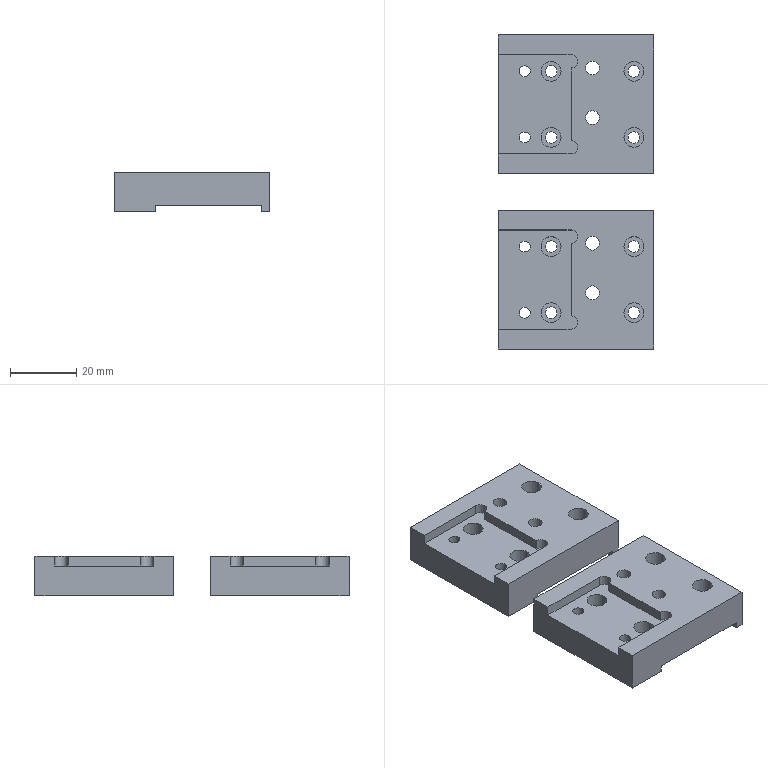NC program | NX | posted with a generic post | part box 47 x 95 x 12 mm
Lines 1 to 1782 of 2681, first 1411 of 1766 lines:
N10 G17 G21 G94 G90
(FLOOR_WALL , TOOL : D80)
N12 T19 M6
N14 G54
N16 G17 G0 G90 X92.5 Y0. S6500 M3
N18 G43 Z30. H19
N20 Z3.
N22 G94 G1 Z0. F1500.
N24 X89.5
N26 X-89.5
N28 X-92.5
N30 Z3.
N32 G0 Z30.
N34 M5
(DRILLING , TOOL : D6A45)
N36 T01 M6
N38 G54
N40 G17 G0 G90 X-36.5 Y-15.5 S5000 M3
N42 G43 Z30. H1
N44 G94 G81 G98 Z-1. F350. R3.
N46 Y-7.5
N48 X-37.5 Y5.
N50 X-36.5 Y17.5
N52 X-16.5
N54 X-22.5 Y5.
N56 X-16.5 Y-7.5
N58 Y-15.5
N60 X16.5
N62 Y-7.5
N64 X15.5 Y5.
N66 X16.5 Y17.5
N68 X36.5
N70 X30.5 Y5.
N72 X36.5 Y-7.5
N74 Y-15.5
N76 G80
N78 G0 X36.5 Y-15.5 Z30.
N80 M5
(DRILLING_COPY_COPY , TOOL : 4.2ZT)
N82 T04 M6
N84 G54
N86 G17 G0 G90 X-37.5 Y5. S2000 M3
N88 G43 Z30. H4
N90 G94 G83 G98 Z-12.762 F300. Q2. R3.
N92 X-22.5
N94 X15.5
N96 X30.5
N98 G80
N100 G0 X30.5 Y5. Z30.
N102 M5
(DRILLING_COPY , TOOL : 3.3ZT)
N104 T03 M6
N106 G54
N108 G17 G0 G90 X-36.5 Y-15.5 S2000 M3
N110 G43 Z30. H3
N112 G94 G83 G98 Z-14.491 F200. Q2. R3.
N114 X-16.5
N116 X16.5
N118 X36.5
N120 G80
N122 G0 X36.5 Y-15.5 Z30.
N124 M5
(DRILLING_COPY_COPY_1 , TOOL : 3.5ZT)
N126 T07 M6
N128 G54
N130 G17 G0 G90 X-16.5 Y-7.5 S2000 M3
N132 G43 Z30. H7
N134 G94 G83 G98 Z-14.052 F200. Q2. R3.
N136 X-36.5
N138 Y17.5
N140 X-16.5
N142 X16.5
N144 X36.5
N146 Y-7.5
N148 X16.5
N150 G80
N152 G0 X16.5 Y-7.5 Z30.
N154 M5
(ZLEVEL_PROFILE , TOOL : D10)
N156 T15 M6
N158 G54
N160 G17 G0 G90 X-0.4 Y-4.832 S9500 M3
N162 G43 Z30. H15
N164 Z1.5
N166 G94 G1 Y-24.054 Z0.493 F1000.
N168 X-0.734 Y-25.398 Z0.42
N170 X-1.416 Y-26.604 Z0.347
N172 X-2.396 Y-27.584 Z0.275
N174 X-3.602 Y-28.266 Z0.202
N176 X-4.946 Y-28.6 Z0.13
N178 X-26.5 Z-1.
N180 X-47.5 F3000.
N182 G2 X-52.6 Y-23.5 R5.1
N184 G1 Y23.5
N186 G2 X-47.5 Y28.6 R5.1
N188 G1 X-5.5
N190 G2 X-0.4 Y23.5 R5.1
N192 G1 Y-23.5
N194 G2 X-5.5 Y-28.6 R5.1
N196 G1 X-26.5
N198 X-47.5 Z-1.1
N200 X-48. Y-28.575 Z-1.102
N202 X-48.495 Y-28.502 Z-1.105
N204 X-48.98 Y-28.38 Z-1.107
N206 X-49.452 Y-28.212 Z-1.11
N208 X-49.904 Y-27.998 Z-1.112
N210 X-50.333 Y-27.74 Z-1.114
N212 X-50.735 Y-27.442 Z-1.117
N214 X-51.106 Y-27.106 Z-1.119
N216 X-51.442 Y-26.735 Z-1.121
N218 X-51.74 Y-26.333 Z-1.124
N220 X-51.998 Y-25.904 Z-1.126
N222 X-52.212 Y-25.452 Z-1.129
N224 X-52.38 Y-24.98 Z-1.131
N226 X-52.502 Y-24.495 Z-1.133
N228 X-52.575 Y-24. Z-1.136
N230 X-52.6 Y-23.5 Z-1.138
N232 Y23.5 Z-1.362
N234 X-52.575 Y24. Z-1.364
N236 X-52.502 Y24.495 Z-1.367
N238 X-52.38 Y24.98 Z-1.369
N240 X-52.212 Y25.452 Z-1.371
N242 X-51.998 Y25.904 Z-1.374
N244 X-51.74 Y26.333 Z-1.376
N246 X-51.442 Y26.735 Z-1.379
N248 X-51.106 Y27.106 Z-1.381
N250 X-50.735 Y27.442 Z-1.383
N252 X-50.333 Y27.74 Z-1.386
N254 X-49.904 Y27.998 Z-1.388
N256 X-49.452 Y28.212 Z-1.39
N258 X-48.98 Y28.38 Z-1.393
N260 X-48.495 Y28.502 Z-1.395
N262 X-48. Y28.575 Z-1.398
N264 X-47.5 Y28.6 Z-1.4
N266 X-5.5 Z-1.6
N268 X-5. Y28.575 Z-1.602
N270 X-4.505 Y28.502 Z-1.605
N272 X-4.02 Y28.38 Z-1.607
N274 X-3.548 Y28.212 Z-1.61
N276 X-3.096 Y27.998 Z-1.612
N278 X-2.667 Y27.74 Z-1.614
N280 X-2.265 Y27.442 Z-1.617
N282 X-1.894 Y27.106 Z-1.619
N284 X-1.558 Y26.735 Z-1.621
N286 X-1.26 Y26.333 Z-1.624
N288 X-1.002 Y25.904 Z-1.626
N290 X-0.788 Y25.452 Z-1.629
N292 X-0.62 Y24.98 Z-1.631
N294 X-0.498 Y24.495 Z-1.633
N296 X-0.425 Y24. Z-1.636
N298 X-0.4 Y23.5 Z-1.638
N300 Y-23.5 Z-1.862
N302 X-0.425 Y-24. Z-1.864
N304 X-0.498 Y-24.495 Z-1.867
N306 X-0.62 Y-24.98 Z-1.869
N308 X-0.788 Y-25.452 Z-1.871
N310 X-1.002 Y-25.904 Z-1.874
N312 X-1.26 Y-26.333 Z-1.876
N314 X-1.558 Y-26.735 Z-1.879
N316 X-1.894 Y-27.106 Z-1.881
N318 X-2.265 Y-27.442 Z-1.883
N320 X-2.667 Y-27.74 Z-1.886
N322 X-3.096 Y-27.998 Z-1.888
N324 X-3.548 Y-28.212 Z-1.89
N326 X-4.02 Y-28.38 Z-1.893
N328 X-4.505 Y-28.502 Z-1.895
N330 X-5. Y-28.575 Z-1.898
N332 X-5.5 Y-28.6 Z-1.9
N334 X-26.5 Z-2.
N336 X-47.5 Z-2.1
N338 X-48. Y-28.575 Z-2.102
N340 X-48.495 Y-28.502 Z-2.105
N342 X-48.98 Y-28.38 Z-2.107
N344 X-49.452 Y-28.212 Z-2.11
N346 X-49.904 Y-27.998 Z-2.112
N348 X-50.333 Y-27.74 Z-2.114
N350 X-50.735 Y-27.442 Z-2.117
N352 X-51.106 Y-27.106 Z-2.119
N354 X-51.442 Y-26.735 Z-2.121
N356 X-51.74 Y-26.333 Z-2.124
N358 X-51.998 Y-25.904 Z-2.126
N360 X-52.212 Y-25.452 Z-2.129
N362 X-52.38 Y-24.98 Z-2.131
N364 X-52.502 Y-24.495 Z-2.133
N366 X-52.575 Y-24. Z-2.136
N368 X-52.6 Y-23.5 Z-2.138
N370 Y23.5 Z-2.362
N372 X-52.575 Y24. Z-2.364
N374 X-52.502 Y24.495 Z-2.367
N376 X-52.38 Y24.98 Z-2.369
N378 X-52.212 Y25.452 Z-2.371
N380 X-51.998 Y25.904 Z-2.374
N382 X-51.74 Y26.333 Z-2.376
N384 X-51.442 Y26.735 Z-2.379
N386 X-51.106 Y27.106 Z-2.381
N388 X-50.735 Y27.442 Z-2.383
N390 X-50.333 Y27.74 Z-2.386
N392 X-49.904 Y27.998 Z-2.388
N394 X-49.452 Y28.212 Z-2.39
N396 X-48.98 Y28.38 Z-2.393
N398 X-48.495 Y28.502 Z-2.395
N400 X-48. Y28.575 Z-2.398
N402 X-47.5 Y28.6 Z-2.4
N404 X-5.5 Z-2.6
N406 X-5. Y28.575 Z-2.602
N408 X-4.505 Y28.502 Z-2.605
N410 X-4.02 Y28.38 Z-2.607
N412 X-3.548 Y28.212 Z-2.61
N414 X-3.096 Y27.998 Z-2.612
N416 X-2.667 Y27.74 Z-2.614
N418 X-2.265 Y27.442 Z-2.617
N420 X-1.894 Y27.106 Z-2.619
N422 X-1.558 Y26.735 Z-2.621
N424 X-1.26 Y26.333 Z-2.624
N426 X-1.002 Y25.904 Z-2.626
N428 X-0.788 Y25.452 Z-2.629
N430 X-0.62 Y24.98 Z-2.631
N432 X-0.498 Y24.495 Z-2.633
N434 X-0.425 Y24. Z-2.636
N436 X-0.4 Y23.5 Z-2.638
N438 Y-23.5 Z-2.862
N440 X-0.425 Y-24. Z-2.864
N442 X-0.498 Y-24.495 Z-2.867
N444 X-0.62 Y-24.98 Z-2.869
N446 X-0.788 Y-25.452 Z-2.871
N448 X-1.002 Y-25.904 Z-2.874
N450 X-1.26 Y-26.333 Z-2.876
N452 X-1.558 Y-26.735 Z-2.879
N454 X-1.894 Y-27.106 Z-2.881
N456 X-2.265 Y-27.442 Z-2.883
N458 X-2.667 Y-27.74 Z-2.886
N460 X-3.096 Y-27.998 Z-2.888
N462 X-3.548 Y-28.212 Z-2.89
N464 X-4.02 Y-28.38 Z-2.893
N466 X-4.505 Y-28.502 Z-2.895
N468 X-5. Y-28.575 Z-2.898
N470 X-5.5 Y-28.6 Z-2.9
N472 X-26.5 Z-3.
N474 X-47.5 Z-3.1
N476 X-48. Y-28.575 Z-3.102
N478 X-48.495 Y-28.502 Z-3.105
N480 X-48.98 Y-28.38 Z-3.107
N482 X-49.452 Y-28.212 Z-3.11
N484 X-49.904 Y-27.998 Z-3.112
N486 X-50.333 Y-27.74 Z-3.114
N488 X-50.735 Y-27.442 Z-3.117
N490 X-51.106 Y-27.106 Z-3.119
N492 X-51.442 Y-26.735 Z-3.121
N494 X-51.74 Y-26.333 Z-3.124
N496 X-51.998 Y-25.904 Z-3.126
N498 X-52.212 Y-25.452 Z-3.129
N500 X-52.38 Y-24.98 Z-3.131
N502 X-52.502 Y-24.495 Z-3.133
N504 X-52.575 Y-24. Z-3.136
N506 X-52.6 Y-23.5 Z-3.138
N508 Y23.5 Z-3.362
N510 X-52.575 Y24. Z-3.364
N512 X-52.502 Y24.495 Z-3.367
N514 X-52.38 Y24.98 Z-3.369
N516 X-52.212 Y25.452 Z-3.371
N518 X-51.998 Y25.904 Z-3.374
N520 X-51.74 Y26.333 Z-3.376
N522 X-51.442 Y26.735 Z-3.379
N524 X-51.106 Y27.106 Z-3.381
N526 X-50.735 Y27.442 Z-3.383
N528 X-50.333 Y27.74 Z-3.386
N530 X-49.904 Y27.998 Z-3.388
N532 X-49.452 Y28.212 Z-3.39
N534 X-48.98 Y28.38 Z-3.393
N536 X-48.495 Y28.502 Z-3.395
N538 X-48. Y28.575 Z-3.398
N540 X-47.5 Y28.6 Z-3.4
N542 X-5.5 Z-3.6
N544 X-5. Y28.575 Z-3.602
N546 X-4.505 Y28.502 Z-3.605
N548 X-4.02 Y28.38 Z-3.607
N550 X-3.548 Y28.212 Z-3.61
N552 X-3.096 Y27.998 Z-3.612
N554 X-2.667 Y27.74 Z-3.614
N556 X-2.265 Y27.442 Z-3.617
N558 X-1.894 Y27.106 Z-3.619
N560 X-1.558 Y26.735 Z-3.621
N562 X-1.26 Y26.333 Z-3.624
N564 X-1.002 Y25.904 Z-3.626
N566 X-0.788 Y25.452 Z-3.629
N568 X-0.62 Y24.98 Z-3.631
N570 X-0.498 Y24.495 Z-3.633
N572 X-0.425 Y24. Z-3.636
N574 X-0.4 Y23.5 Z-3.638
N576 Y-23.5 Z-3.862
N578 X-0.425 Y-24. Z-3.864
N580 X-0.498 Y-24.495 Z-3.867
N582 X-0.62 Y-24.98 Z-3.869
N584 X-0.788 Y-25.452 Z-3.871
N586 X-1.002 Y-25.904 Z-3.874
N588 X-1.26 Y-26.333 Z-3.876
N590 X-1.558 Y-26.735 Z-3.879
N592 X-1.894 Y-27.106 Z-3.881
N594 X-2.265 Y-27.442 Z-3.883
N596 X-2.667 Y-27.74 Z-3.886
N598 X-3.096 Y-27.998 Z-3.888
N600 X-3.548 Y-28.212 Z-3.89
N602 X-4.02 Y-28.38 Z-3.893
N604 X-4.505 Y-28.502 Z-3.895
N606 X-5. Y-28.575 Z-3.898
N608 X-5.5 Y-28.6 Z-3.9
N610 X-26.5 Z-4.
N612 X-47.5 Z-4.1
N614 X-48. Y-28.575 Z-4.102
N616 X-48.495 Y-28.502 Z-4.105
N618 X-48.98 Y-28.38 Z-4.107
N620 X-49.452 Y-28.212 Z-4.11
N622 X-49.904 Y-27.998 Z-4.112
N624 X-50.333 Y-27.74 Z-4.114
N626 X-50.735 Y-27.442 Z-4.117
N628 X-51.106 Y-27.106 Z-4.119
N630 X-51.442 Y-26.735 Z-4.121
N632 X-51.74 Y-26.333 Z-4.124
N634 X-51.998 Y-25.904 Z-4.126
N636 X-52.212 Y-25.452 Z-4.129
N638 X-52.38 Y-24.98 Z-4.131
N640 X-52.502 Y-24.495 Z-4.133
N642 X-52.575 Y-24. Z-4.136
N644 X-52.6 Y-23.5 Z-4.138
N646 Y23.5 Z-4.362
N648 X-52.575 Y24. Z-4.364
N650 X-52.502 Y24.495 Z-4.367
N652 X-52.38 Y24.98 Z-4.369
N654 X-52.212 Y25.452 Z-4.371
N656 X-51.998 Y25.904 Z-4.374
N658 X-51.74 Y26.333 Z-4.376
N660 X-51.442 Y26.735 Z-4.379
N662 X-51.106 Y27.106 Z-4.381
N664 X-50.735 Y27.442 Z-4.383
N666 X-50.333 Y27.74 Z-4.386
N668 X-49.904 Y27.998 Z-4.388
N670 X-49.452 Y28.212 Z-4.39
N672 X-48.98 Y28.38 Z-4.393
N674 X-48.495 Y28.502 Z-4.395
N676 X-48. Y28.575 Z-4.398
N678 X-47.5 Y28.6 Z-4.4
N680 X-5.5 Z-4.6
N682 X-5. Y28.575 Z-4.602
N684 X-4.505 Y28.502 Z-4.605
N686 X-4.02 Y28.38 Z-4.607
N688 X-3.548 Y28.212 Z-4.61
N690 X-3.096 Y27.998 Z-4.612
N692 X-2.667 Y27.74 Z-4.614
N694 X-2.265 Y27.442 Z-4.617
N696 X-1.894 Y27.106 Z-4.619
N698 X-1.558 Y26.735 Z-4.621
N700 X-1.26 Y26.333 Z-4.624
N702 X-1.002 Y25.904 Z-4.626
N704 X-0.788 Y25.452 Z-4.629
N706 X-0.62 Y24.98 Z-4.631
N708 X-0.498 Y24.495 Z-4.633
N710 X-0.425 Y24. Z-4.636
N712 X-0.4 Y23.5 Z-4.638
N714 Y-23.5 Z-4.862
N716 X-0.425 Y-24. Z-4.864
N718 X-0.498 Y-24.495 Z-4.867
N720 X-0.62 Y-24.98 Z-4.869
N722 X-0.788 Y-25.452 Z-4.871
N724 X-1.002 Y-25.904 Z-4.874
N726 X-1.26 Y-26.333 Z-4.876
N728 X-1.558 Y-26.735 Z-4.879
N730 X-1.894 Y-27.106 Z-4.881
N732 X-2.265 Y-27.442 Z-4.883
N734 X-2.667 Y-27.74 Z-4.886
N736 X-3.096 Y-27.998 Z-4.888
N738 X-3.548 Y-28.212 Z-4.89
N740 X-4.02 Y-28.38 Z-4.893
N742 X-4.505 Y-28.502 Z-4.895
N744 X-5. Y-28.575 Z-4.898
N746 X-5.5 Y-28.6 Z-4.9
N748 X-26.5 Z-5.
N750 X-47.5 Z-5.1
N752 X-48. Y-28.575 Z-5.102
N754 X-48.495 Y-28.502 Z-5.105
N756 X-48.98 Y-28.38 Z-5.107
N758 X-49.452 Y-28.212 Z-5.11
N760 X-49.904 Y-27.998 Z-5.112
N762 X-50.333 Y-27.74 Z-5.114
N764 X-50.735 Y-27.442 Z-5.117
N766 X-51.106 Y-27.106 Z-5.119
N768 X-51.442 Y-26.735 Z-5.121
N770 X-51.74 Y-26.333 Z-5.124
N772 X-51.998 Y-25.904 Z-5.126
N774 X-52.212 Y-25.452 Z-5.129
N776 X-52.38 Y-24.98 Z-5.131
N778 X-52.502 Y-24.495 Z-5.133
N780 X-52.575 Y-24. Z-5.136
N782 X-52.6 Y-23.5 Z-5.138
N784 Y23.5 Z-5.362
N786 X-52.575 Y24. Z-5.364
N788 X-52.502 Y24.495 Z-5.367
N790 X-52.38 Y24.98 Z-5.369
N792 X-52.212 Y25.452 Z-5.371
N794 X-51.998 Y25.904 Z-5.374
N796 X-51.74 Y26.333 Z-5.376
N798 X-51.442 Y26.735 Z-5.379
N800 X-51.106 Y27.106 Z-5.381
N802 X-50.735 Y27.442 Z-5.383
N804 X-50.333 Y27.74 Z-5.386
N806 X-49.904 Y27.998 Z-5.388
N808 X-49.452 Y28.212 Z-5.39
N810 X-48.98 Y28.38 Z-5.393
N812 X-48.495 Y28.502 Z-5.395
N814 X-48. Y28.575 Z-5.398
N816 X-47.5 Y28.6 Z-5.4
N818 X-5.5 Z-5.6
N820 X-5. Y28.575 Z-5.602
N822 X-4.505 Y28.502 Z-5.605
N824 X-4.02 Y28.38 Z-5.607
N826 X-3.548 Y28.212 Z-5.61
N828 X-3.096 Y27.998 Z-5.612
N830 X-2.667 Y27.74 Z-5.614
N832 X-2.265 Y27.442 Z-5.617
N834 X-1.894 Y27.106 Z-5.619
N836 X-1.558 Y26.735 Z-5.621
N838 X-1.26 Y26.333 Z-5.624
N840 X-1.002 Y25.904 Z-5.626
N842 X-0.788 Y25.452 Z-5.629
N844 X-0.62 Y24.98 Z-5.631
N846 X-0.498 Y24.495 Z-5.633
N848 X-0.425 Y24. Z-5.636
N850 X-0.4 Y23.5 Z-5.638
N852 Y-23.5 Z-5.862
N854 X-0.425 Y-24. Z-5.864
N856 X-0.498 Y-24.495 Z-5.867
N858 X-0.62 Y-24.98 Z-5.869
N860 X-0.788 Y-25.452 Z-5.871
N862 X-1.002 Y-25.904 Z-5.874
N864 X-1.26 Y-26.333 Z-5.876
N866 X-1.558 Y-26.735 Z-5.879
N868 X-1.894 Y-27.106 Z-5.881
N870 X-2.265 Y-27.442 Z-5.883
N872 X-2.667 Y-27.74 Z-5.886
N874 X-3.096 Y-27.998 Z-5.888
N876 X-3.548 Y-28.212 Z-5.89
N878 X-4.02 Y-28.38 Z-5.893
N880 X-4.505 Y-28.502 Z-5.895
N882 X-5. Y-28.575 Z-5.898
N884 X-5.5 Y-28.6 Z-5.9
N886 X-26.5 Z-6.
N888 X-47.5 Z-6.1
N890 X-48. Y-28.575 Z-6.102
N892 X-48.495 Y-28.502 Z-6.105
N894 X-48.98 Y-28.38 Z-6.107
N896 X-49.452 Y-28.212 Z-6.11
N898 X-49.904 Y-27.998 Z-6.112
N900 X-50.333 Y-27.74 Z-6.114
N902 X-50.735 Y-27.442 Z-6.117
N904 X-51.106 Y-27.106 Z-6.119
N906 X-51.442 Y-26.735 Z-6.121
N908 X-51.74 Y-26.333 Z-6.124
N910 X-51.998 Y-25.904 Z-6.126
N912 X-52.212 Y-25.452 Z-6.129
N914 X-52.38 Y-24.98 Z-6.131
N916 X-52.502 Y-24.495 Z-6.133
N918 X-52.575 Y-24. Z-6.136
N920 X-52.6 Y-23.5 Z-6.138
N922 Y23.5 Z-6.362
N924 X-52.575 Y24. Z-6.364
N926 X-52.502 Y24.495 Z-6.367
N928 X-52.38 Y24.98 Z-6.369
N930 X-52.212 Y25.452 Z-6.371
N932 X-51.998 Y25.904 Z-6.374
N934 X-51.74 Y26.333 Z-6.376
N936 X-51.442 Y26.735 Z-6.379
N938 X-51.106 Y27.106 Z-6.381
N940 X-50.735 Y27.442 Z-6.383
N942 X-50.333 Y27.74 Z-6.386
N944 X-49.904 Y27.998 Z-6.388
N946 X-49.452 Y28.212 Z-6.39
N948 X-48.98 Y28.38 Z-6.393
N950 X-48.495 Y28.502 Z-6.395
N952 X-48. Y28.575 Z-6.398
N954 X-47.5 Y28.6 Z-6.4
N956 X-5.5 Z-6.6
N958 X-5. Y28.575 Z-6.602
N960 X-4.505 Y28.502 Z-6.605
N962 X-4.02 Y28.38 Z-6.607
N964 X-3.548 Y28.212 Z-6.61
N966 X-3.096 Y27.998 Z-6.612
N968 X-2.667 Y27.74 Z-6.614
N970 X-2.265 Y27.442 Z-6.617
N972 X-1.894 Y27.106 Z-6.619
N974 X-1.558 Y26.735 Z-6.621
N976 X-1.26 Y26.333 Z-6.624
N978 X-1.002 Y25.904 Z-6.626
N980 X-0.788 Y25.452 Z-6.629
N982 X-0.62 Y24.98 Z-6.631
N984 X-0.498 Y24.495 Z-6.633
N986 X-0.425 Y24. Z-6.636
N988 X-0.4 Y23.5 Z-6.638
N990 Y-23.5 Z-6.862
N992 X-0.425 Y-24. Z-6.864
N994 X-0.498 Y-24.495 Z-6.867
N996 X-0.62 Y-24.98 Z-6.869
N998 X-0.788 Y-25.452 Z-6.871
N1000 X-1.002 Y-25.904 Z-6.874
N1002 X-1.26 Y-26.333 Z-6.876
N1004 X-1.558 Y-26.735 Z-6.879
N1006 X-1.894 Y-27.106 Z-6.881
N1008 X-2.265 Y-27.442 Z-6.883
N1010 X-2.667 Y-27.74 Z-6.886
N1012 X-3.096 Y-27.998 Z-6.888
N1014 X-3.548 Y-28.212 Z-6.89
N1016 X-4.02 Y-28.38 Z-6.893
N1018 X-4.505 Y-28.502 Z-6.895
N1020 X-5. Y-28.575 Z-6.898
N1022 X-5.5 Y-28.6 Z-6.9
N1024 X-26.5 Z-7.
N1026 X-47.5 Z-7.1
N1028 X-48. Y-28.575 Z-7.102
N1030 X-48.495 Y-28.502 Z-7.105
N1032 X-48.98 Y-28.38 Z-7.107
N1034 X-49.452 Y-28.212 Z-7.11
N1036 X-49.904 Y-27.998 Z-7.112
N1038 X-50.333 Y-27.74 Z-7.114
N1040 X-50.735 Y-27.442 Z-7.117
N1042 X-51.106 Y-27.106 Z-7.119
N1044 X-51.442 Y-26.735 Z-7.121
N1046 X-51.74 Y-26.333 Z-7.124
N1048 X-51.998 Y-25.904 Z-7.126
N1050 X-52.212 Y-25.452 Z-7.129
N1052 X-52.38 Y-24.98 Z-7.131
N1054 X-52.502 Y-24.495 Z-7.133
N1056 X-52.575 Y-24. Z-7.136
N1058 X-52.6 Y-23.5 Z-7.138
N1060 Y23.5 Z-7.362
N1062 X-52.575 Y24. Z-7.364
N1064 X-52.502 Y24.495 Z-7.367
N1066 X-52.38 Y24.98 Z-7.369
N1068 X-52.212 Y25.452 Z-7.371
N1070 X-51.998 Y25.904 Z-7.374
N1072 X-51.74 Y26.333 Z-7.376
N1074 X-51.442 Y26.735 Z-7.379
N1076 X-51.106 Y27.106 Z-7.381
N1078 X-50.735 Y27.442 Z-7.383
N1080 X-50.333 Y27.74 Z-7.386
N1082 X-49.904 Y27.998 Z-7.388
N1084 X-49.452 Y28.212 Z-7.39
N1086 X-48.98 Y28.38 Z-7.393
N1088 X-48.495 Y28.502 Z-7.395
N1090 X-48. Y28.575 Z-7.398
N1092 X-47.5 Y28.6 Z-7.4
N1094 X-5.5 Z-7.6
N1096 X-5. Y28.575 Z-7.602
N1098 X-4.505 Y28.502 Z-7.605
N1100 X-4.02 Y28.38 Z-7.607
N1102 X-3.548 Y28.212 Z-7.61
N1104 X-3.096 Y27.998 Z-7.612
N1106 X-2.667 Y27.74 Z-7.614
N1108 X-2.265 Y27.442 Z-7.617
N1110 X-1.894 Y27.106 Z-7.619
N1112 X-1.558 Y26.735 Z-7.621
N1114 X-1.26 Y26.333 Z-7.624
N1116 X-1.002 Y25.904 Z-7.626
N1118 X-0.788 Y25.452 Z-7.629
N1120 X-0.62 Y24.98 Z-7.631
N1122 X-0.498 Y24.495 Z-7.633
N1124 X-0.425 Y24. Z-7.636
N1126 X-0.4 Y23.5 Z-7.638
N1128 Y-23.5 Z-7.862
N1130 X-0.425 Y-24. Z-7.864
N1132 X-0.498 Y-24.495 Z-7.867
N1134 X-0.62 Y-24.98 Z-7.869
N1136 X-0.788 Y-25.452 Z-7.871
N1138 X-1.002 Y-25.904 Z-7.874
N1140 X-1.26 Y-26.333 Z-7.876
N1142 X-1.558 Y-26.735 Z-7.879
N1144 X-1.894 Y-27.106 Z-7.881
N1146 X-2.265 Y-27.442 Z-7.883
N1148 X-2.667 Y-27.74 Z-7.886
N1150 X-3.096 Y-27.998 Z-7.888
N1152 X-3.548 Y-28.212 Z-7.89
N1154 X-4.02 Y-28.38 Z-7.893
N1156 X-4.505 Y-28.502 Z-7.895
N1158 X-5. Y-28.575 Z-7.898
N1160 X-5.5 Y-28.6 Z-7.9
N1162 X-26.5 Z-8.
N1164 X-47.5 Z-8.1
N1166 X-48. Y-28.575 Z-8.102
N1168 X-48.495 Y-28.502 Z-8.105
N1170 X-48.98 Y-28.38 Z-8.107
N1172 X-49.452 Y-28.212 Z-8.11
N1174 X-49.904 Y-27.998 Z-8.112
N1176 X-50.333 Y-27.74 Z-8.114
N1178 X-50.735 Y-27.442 Z-8.117
N1180 X-51.106 Y-27.106 Z-8.119
N1182 X-51.442 Y-26.735 Z-8.121
N1184 X-51.74 Y-26.333 Z-8.124
N1186 X-51.998 Y-25.904 Z-8.126
N1188 X-52.212 Y-25.452 Z-8.129
N1190 X-52.38 Y-24.98 Z-8.131
N1192 X-52.502 Y-24.495 Z-8.133
N1194 X-52.575 Y-24. Z-8.136
N1196 X-52.6 Y-23.5 Z-8.138
N1198 Y23.5 Z-8.362
N1200 X-52.575 Y24. Z-8.364
N1202 X-52.502 Y24.495 Z-8.367
N1204 X-52.38 Y24.98 Z-8.369
N1206 X-52.212 Y25.452 Z-8.371
N1208 X-51.998 Y25.904 Z-8.374
N1210 X-51.74 Y26.333 Z-8.376
N1212 X-51.442 Y26.735 Z-8.379
N1214 X-51.106 Y27.106 Z-8.381
N1216 X-50.735 Y27.442 Z-8.383
N1218 X-50.333 Y27.74 Z-8.386
N1220 X-49.904 Y27.998 Z-8.388
N1222 X-49.452 Y28.212 Z-8.39
N1224 X-48.98 Y28.38 Z-8.393
N1226 X-48.495 Y28.502 Z-8.395
N1228 X-48. Y28.575 Z-8.398
N1230 X-47.5 Y28.6 Z-8.4
N1232 X-5.5 Z-8.6
N1234 X-5. Y28.575 Z-8.602
N1236 X-4.505 Y28.502 Z-8.605
N1238 X-4.02 Y28.38 Z-8.607
N1240 X-3.548 Y28.212 Z-8.61
N1242 X-3.096 Y27.998 Z-8.612
N1244 X-2.667 Y27.74 Z-8.614
N1246 X-2.265 Y27.442 Z-8.617
N1248 X-1.894 Y27.106 Z-8.619
N1250 X-1.558 Y26.735 Z-8.621
N1252 X-1.26 Y26.333 Z-8.624
N1254 X-1.002 Y25.904 Z-8.626
N1256 X-0.788 Y25.452 Z-8.629
N1258 X-0.62 Y24.98 Z-8.631
N1260 X-0.498 Y24.495 Z-8.633
N1262 X-0.425 Y24. Z-8.636
N1264 X-0.4 Y23.5 Z-8.638
N1266 Y-23.5 Z-8.862
N1268 X-0.425 Y-24. Z-8.864
N1270 X-0.498 Y-24.495 Z-8.867
N1272 X-0.62 Y-24.98 Z-8.869
N1274 X-0.788 Y-25.452 Z-8.871
N1276 X-1.002 Y-25.904 Z-8.874
N1278 X-1.26 Y-26.333 Z-8.876
N1280 X-1.558 Y-26.735 Z-8.879
N1282 X-1.894 Y-27.106 Z-8.881
N1284 X-2.265 Y-27.442 Z-8.883
N1286 X-2.667 Y-27.74 Z-8.886
N1288 X-3.096 Y-27.998 Z-8.888
N1290 X-3.548 Y-28.212 Z-8.89
N1292 X-4.02 Y-28.38 Z-8.893
N1294 X-4.505 Y-28.502 Z-8.895
N1296 X-5. Y-28.575 Z-8.898
N1298 X-5.5 Y-28.6 Z-8.9
N1300 X-26.5 Z-9.
N1302 X-47.5 Z-9.1
N1304 X-48. Y-28.575 Z-9.102
N1306 X-48.495 Y-28.502 Z-9.105
N1308 X-48.98 Y-28.38 Z-9.107
N1310 X-49.452 Y-28.212 Z-9.11
N1312 X-49.904 Y-27.998 Z-9.112
N1314 X-50.333 Y-27.74 Z-9.114
N1316 X-50.735 Y-27.442 Z-9.117
N1318 X-51.106 Y-27.106 Z-9.119
N1320 X-51.442 Y-26.735 Z-9.121
N1322 X-51.74 Y-26.333 Z-9.124
N1324 X-51.998 Y-25.904 Z-9.126
N1326 X-52.212 Y-25.452 Z-9.129
N1328 X-52.38 Y-24.98 Z-9.131
N1330 X-52.502 Y-24.495 Z-9.133
N1332 X-52.575 Y-24. Z-9.136
N1334 X-52.6 Y-23.5 Z-9.138
N1336 Y23.5 Z-9.362
N1338 X-52.575 Y24. Z-9.364
N1340 X-52.502 Y24.495 Z-9.367
N1342 X-52.38 Y24.98 Z-9.369
N1344 X-52.212 Y25.452 Z-9.371
N1346 X-51.998 Y25.904 Z-9.374
N1348 X-51.74 Y26.333 Z-9.376
N1350 X-51.442 Y26.735 Z-9.379
N1352 X-51.106 Y27.106 Z-9.381
N1354 X-50.735 Y27.442 Z-9.383
N1356 X-50.333 Y27.74 Z-9.386
N1358 X-49.904 Y27.998 Z-9.388
N1360 X-49.452 Y28.212 Z-9.39
N1362 X-48.98 Y28.38 Z-9.393
N1364 X-48.495 Y28.502 Z-9.395
N1366 X-48. Y28.575 Z-9.398
N1368 X-47.5 Y28.6 Z-9.4
N1370 X-5.5 Z-9.6
N1372 X-5. Y28.575 Z-9.602
N1374 X-4.505 Y28.502 Z-9.605
N1376 X-4.02 Y28.38 Z-9.607
N1378 X-3.548 Y28.212 Z-9.61
N1380 X-3.096 Y27.998 Z-9.612
N1382 X-2.667 Y27.74 Z-9.614
N1384 X-2.265 Y27.442 Z-9.617
N1386 X-1.894 Y27.106 Z-9.619
N1388 X-1.558 Y26.735 Z-9.621
N1390 X-1.26 Y26.333 Z-9.624
N1392 X-1.002 Y25.904 Z-9.626
N1394 X-0.788 Y25.452 Z-9.629
N1396 X-0.62 Y24.98 Z-9.631
N1398 X-0.498 Y24.495 Z-9.633
N1400 X-0.425 Y24. Z-9.636
N1402 X-0.4 Y23.5 Z-9.638
N1404 Y-23.5 Z-9.862
N1406 X-0.425 Y-24. Z-9.864
N1408 X-0.498 Y-24.495 Z-9.867
N1410 X-0.62 Y-24.98 Z-9.869
N1412 X-0.788 Y-25.452 Z-9.871
N1414 X-1.002 Y-25.904 Z-9.874
N1416 X-1.26 Y-26.333 Z-9.876
N1418 X-1.558 Y-26.735 Z-9.879
N1420 X-1.894 Y-27.106 Z-9.881
N1422 X-2.265 Y-27.442 Z-9.883
N1424 X-2.667 Y-27.74 Z-9.886
N1426 X-3.096 Y-27.998 Z-9.888
N1428 X-3.548 Y-28.212 Z-9.89
N1430 X-4.02 Y-28.38 Z-9.893
N1432 X-4.505 Y-28.502 Z-9.895
N1434 X-5. Y-28.575 Z-9.898
N1436 X-5.5 Y-28.6 Z-9.9
N1438 X-26.5 Z-10.
N1440 X-47.5 Z-10.1
N1442 X-48. Y-28.575 Z-10.102
N1444 X-48.495 Y-28.502 Z-10.105
N1446 X-48.98 Y-28.38 Z-10.107
N1448 X-49.452 Y-28.212 Z-10.11
N1450 X-49.904 Y-27.998 Z-10.112
N1452 X-50.333 Y-27.74 Z-10.114
N1454 X-50.735 Y-27.442 Z-10.117
N1456 X-51.106 Y-27.106 Z-10.119
N1458 X-51.442 Y-26.735 Z-10.121
N1460 X-51.74 Y-26.333 Z-10.124
N1462 X-51.998 Y-25.904 Z-10.126
N1464 X-52.212 Y-25.452 Z-10.129
N1466 X-52.38 Y-24.98 Z-10.131
N1468 X-52.502 Y-24.495 Z-10.133
N1470 X-52.575 Y-24. Z-10.136
N1472 X-52.6 Y-23.5 Z-10.138
N1474 Y23.5 Z-10.362
N1476 X-52.575 Y24. Z-10.364
N1478 X-52.502 Y24.495 Z-10.367
N1480 X-52.38 Y24.98 Z-10.369
N1482 X-52.212 Y25.452 Z-10.371
N1484 X-51.998 Y25.904 Z-10.374
N1486 X-51.74 Y26.333 Z-10.376
N1488 X-51.442 Y26.735 Z-10.379
N1490 X-51.106 Y27.106 Z-10.381
N1492 X-50.735 Y27.442 Z-10.383
N1494 X-50.333 Y27.74 Z-10.386
N1496 X-49.904 Y27.998 Z-10.388
N1498 X-49.452 Y28.212 Z-10.39
N1500 X-48.98 Y28.38 Z-10.393
N1502 X-48.495 Y28.502 Z-10.395
N1504 X-48. Y28.575 Z-10.398
N1506 X-47.5 Y28.6 Z-10.4
N1508 X-5.5 Z-10.6
N1510 X-5. Y28.575 Z-10.602
N1512 X-4.505 Y28.502 Z-10.605
N1514 X-4.02 Y28.38 Z-10.607
N1516 X-3.548 Y28.212 Z-10.61
N1518 X-3.096 Y27.998 Z-10.612
N1520 X-2.667 Y27.74 Z-10.614
N1522 X-2.265 Y27.442 Z-10.617
N1524 X-1.894 Y27.106 Z-10.619
N1526 X-1.558 Y26.735 Z-10.621
N1528 X-1.26 Y26.333 Z-10.624
N1530 X-1.002 Y25.904 Z-10.626
N1532 X-0.788 Y25.452 Z-10.629
N1534 X-0.62 Y24.98 Z-10.631
N1536 X-0.498 Y24.495 Z-10.633
N1538 X-0.425 Y24. Z-10.636
N1540 X-0.4 Y23.5 Z-10.638
N1542 Y-23.5 Z-10.862
N1544 X-0.425 Y-24. Z-10.864
N1546 X-0.498 Y-24.495 Z-10.867
N1548 X-0.62 Y-24.98 Z-10.869
N1550 X-0.788 Y-25.452 Z-10.871
N1552 X-1.002 Y-25.904 Z-10.874
N1554 X-1.26 Y-26.333 Z-10.876
N1556 X-1.558 Y-26.735 Z-10.879
N1558 X-1.894 Y-27.106 Z-10.881
N1560 X-2.265 Y-27.442 Z-10.883
N1562 X-2.667 Y-27.74 Z-10.886
N1564 X-3.096 Y-27.998 Z-10.888
N1566 X-3.548 Y-28.212 Z-10.89
N1568 X-4.02 Y-28.38 Z-10.893
N1570 X-4.505 Y-28.502 Z-10.895
N1572 X-5. Y-28.575 Z-10.898
N1574 X-5.5 Y-28.6 Z-10.9
N1576 X-26.5 Z-11.
N1578 X-47.5 Z-11.1
N1580 X-48. Y-28.575 Z-11.102
N1582 X-48.495 Y-28.502 Z-11.105
N1584 X-48.98 Y-28.38 Z-11.107
N1586 X-49.452 Y-28.212 Z-11.11
N1588 X-49.904 Y-27.998 Z-11.112
N1590 X-50.333 Y-27.74 Z-11.114
N1592 X-50.735 Y-27.442 Z-11.117
N1594 X-51.106 Y-27.106 Z-11.119
N1596 X-51.442 Y-26.735 Z-11.121
N1598 X-51.74 Y-26.333 Z-11.124
N1600 X-51.998 Y-25.904 Z-11.126
N1602 X-52.212 Y-25.452 Z-11.129
N1604 X-52.38 Y-24.98 Z-11.131
N1606 X-52.502 Y-24.495 Z-11.133
N1608 X-52.575 Y-24. Z-11.136
N1610 X-52.6 Y-23.5 Z-11.138
N1612 Y23.5 Z-11.362
N1614 X-52.575 Y24. Z-11.364
N1616 X-52.502 Y24.495 Z-11.367
N1618 X-52.38 Y24.98 Z-11.369
N1620 X-52.212 Y25.452 Z-11.371
N1622 X-51.998 Y25.904 Z-11.374
N1624 X-51.74 Y26.333 Z-11.376
N1626 X-51.442 Y26.735 Z-11.379
N1628 X-51.106 Y27.106 Z-11.381
N1630 X-50.735 Y27.442 Z-11.383
N1632 X-50.333 Y27.74 Z-11.386
N1634 X-49.904 Y27.998 Z-11.388
N1636 X-49.452 Y28.212 Z-11.39
N1638 X-48.98 Y28.38 Z-11.393
N1640 X-48.495 Y28.502 Z-11.395
N1642 X-48. Y28.575 Z-11.398
N1644 X-47.5 Y28.6 Z-11.4
N1646 X-5.5 Z-11.6
N1648 X-5. Y28.575 Z-11.602
N1650 X-4.505 Y28.502 Z-11.605
N1652 X-4.02 Y28.38 Z-11.607
N1654 X-3.548 Y28.212 Z-11.61
N1656 X-3.096 Y27.998 Z-11.612
N1658 X-2.667 Y27.74 Z-11.614
N1660 X-2.265 Y27.442 Z-11.617
N1662 X-1.894 Y27.106 Z-11.619
N1664 X-1.558 Y26.735 Z-11.621
N1666 X-1.26 Y26.333 Z-11.624
N1668 X-1.002 Y25.904 Z-11.626
N1670 X-0.788 Y25.452 Z-11.629
N1672 X-0.62 Y24.98 Z-11.631
N1674 X-0.498 Y24.495 Z-11.633
N1676 X-0.425 Y24. Z-11.636
N1678 X-0.4 Y23.5 Z-11.638
N1680 Y-23.5 Z-11.862
N1682 X-0.425 Y-24. Z-11.864
N1684 X-0.498 Y-24.495 Z-11.867
N1686 X-0.62 Y-24.98 Z-11.869
N1688 X-0.788 Y-25.452 Z-11.871
N1690 X-1.002 Y-25.904 Z-11.874
N1692 X-1.26 Y-26.333 Z-11.876
N1694 X-1.558 Y-26.735 Z-11.879
N1696 X-1.894 Y-27.106 Z-11.881
N1698 X-2.265 Y-27.442 Z-11.883
N1700 X-2.667 Y-27.74 Z-11.886
N1702 X-3.096 Y-27.998 Z-11.888
N1704 X-3.548 Y-28.212 Z-11.89
N1706 X-4.02 Y-28.38 Z-11.893
N1708 X-4.505 Y-28.502 Z-11.895
N1710 X-5. Y-28.575 Z-11.898
N1712 X-5.5 Y-28.6 Z-11.9
N1714 X-26.5 Z-12.
N1716 X-47.5
N1718 G2 X-52.6 Y-23.5 R5.1
N1720 G1 Y23.5
N1722 G2 X-47.5 Y28.6 R5.1
N1724 G1 X-5.5
N1726 G2 X-0.4 Y23.5 R5.1
N1728 G1 Y-23.5
N1730 G2 X-5.5 Y-28.6 R5.1
N1732 G1 X-26.5
N1734 Z-10.5
N1736 G0 Z53.
N1738 X52.6 Y-4.832
N1740 Z1.5
N1742 G1 Y-24.054 Z0.493 F1000.
N1744 X52.266 Y-25.398 Z0.42
N1746 X51.584 Y-26.604 Z0.347
N1748 X50.604 Y-27.584 Z0.275
N1750 X49.398 Y-28.266 Z0.202
N1752 X48.054 Y-28.6 Z0.13
N1754 X26.5 Z-1.
N1756 X5.5 F3000.
N1758 G2 X0.4 Y-23.5 R5.1
N1760 G1 Y23.5
N1762 G2 X5.5 Y28.6 R5.1
N1764 G1 X47.5
N1766 G2 X52.6 Y23.5 R5.1
N1768 G1 Y-23.5
N1770 G2 X47.5 Y-28.6 R5.1
N1772 G1 X26.5
N1774 X5.5 Z-1.1
N1776 X5. Y-28.575 Z-1.102
N1778 X4.505 Y-28.502 Z-1.105
N1780 X4.02 Y-28.38 Z-1.107
N1782 X3.548 Y-28.212 Z-1.11
N1784 X3.096 Y-27.998 Z-1.112
N1786 X2.667 Y-27.74 Z-1.114
N1788 X2.265 Y-27.442 Z-1.117
N1790 X1.894 Y-27.106 Z-1.119
N1792 X1.558 Y-26.735 Z-1.121
N1794 X1.26 Y-26.333 Z-1.124
N1796 X1.002 Y-25.904 Z-1.126
N1798 X0.788 Y-25.452 Z-1.129
N1800 X0.62 Y-24.98 Z-1.131
N1802 X0.498 Y-24.495 Z-1.133
N1804 X0.425 Y-24. Z-1.136
N1806 X0.4 Y-23.5 Z-1.138
N1808 Y23.5 Z-1.362
N1810 X0.425 Y24. Z-1.364
N1812 X0.498 Y24.495 Z-1.367
N1814 X0.62 Y24.98 Z-1.369
N1816 X0.788 Y25.452 Z-1.371
N1818 X1.002 Y25.904 Z-1.374
N1820 X1.26 Y26.333 Z-1.376
N1822 X1.558 Y26.735 Z-1.379
N1824 X1.894 Y27.106 Z-1.381
N1826 X2.265 Y27.442 Z-1.383
N1828 X2.667 Y27.74 Z-1.386
N1830 X3.096 Y27.998 Z-1.388
N1832 X3.548 Y28.212 Z-1.39
N1834 X4.02 Y28.38 Z-1.393
N1836 X4.505 Y28.502 Z-1.395
N1838 X5. Y28.575 Z-1.398
N1840 X5.5 Y28.6 Z-1.4
N1842 X47.5 Z-1.6
N1844 X48. Y28.575 Z-1.602
N1846 X48.495 Y28.502 Z-1.605
N1848 X48.98 Y28.38 Z-1.607
N1850 X49.452 Y28.212 Z-1.61
N1852 X49.904 Y27.998 Z-1.612
N1854 X50.333 Y27.74 Z-1.614
N1856 X50.735 Y27.442 Z-1.617
N1858 X51.106 Y27.106 Z-1.619
N1860 X51.442 Y26.735 Z-1.621
N1862 X51.74 Y26.333 Z-1.624
N1864 X51.998 Y25.904 Z-1.626
N1866 X52.212 Y25.452 Z-1.629
N1868 X52.38 Y24.98 Z-1.631
N1870 X52.502 Y24.495 Z-1.633
N1872 X52.575 Y24. Z-1.636
N1874 X52.6 Y23.5 Z-1.638
N1876 Y-23.5 Z-1.862
N1878 X52.575 Y-24. Z-1.864
N1880 X52.502 Y-24.495 Z-1.867
N1882 X52.38 Y-24.98 Z-1.869
N1884 X52.212 Y-25.452 Z-1.871
N1886 X51.998 Y-25.904 Z-1.874
N1888 X51.74 Y-26.333 Z-1.876
N1890 X51.442 Y-26.735 Z-1.879
N1892 X51.106 Y-27.106 Z-1.881
N1894 X50.735 Y-27.442 Z-1.883
N1896 X50.333 Y-27.74 Z-1.886
N1898 X49.904 Y-27.998 Z-1.888
N1900 X49.452 Y-28.212 Z-1.89
N1902 X48.98 Y-28.38 Z-1.893
N1904 X48.495 Y-28.502 Z-1.895
N1906 X48. Y-28.575 Z-1.898
N1908 X47.5 Y-28.6 Z-1.9
N1910 X26.5 Z-2.
N1912 X5.5 Z-2.1
N1914 X5. Y-28.575 Z-2.102
N1916 X4.505 Y-28.502 Z-2.105
N1918 X4.02 Y-28.38 Z-2.107
N1920 X3.548 Y-28.212 Z-2.11
N1922 X3.096 Y-27.998 Z-2.112
N1924 X2.667 Y-27.74 Z-2.114
N1926 X2.265 Y-27.442 Z-2.117
N1928 X1.894 Y-27.106 Z-2.119
N1930 X1.558 Y-26.735 Z-2.121
N1932 X1.26 Y-26.333 Z-2.124
N1934 X1.002 Y-25.904 Z-2.126
N1936 X0.788 Y-25.452 Z-2.129
N1938 X0.62 Y-24.98 Z-2.131
N1940 X0.498 Y-24.495 Z-2.133
N1942 X0.425 Y-24. Z-2.136
N1944 X0.4 Y-23.5 Z-2.138
N1946 Y23.5 Z-2.362
N1948 X0.425 Y24. Z-2.364
N1950 X0.498 Y24.495 Z-2.367
N1952 X0.62 Y24.98 Z-2.369
N1954 X0.788 Y25.452 Z-2.371
N1956 X1.002 Y25.904 Z-2.374
N1958 X1.26 Y26.333 Z-2.376
N1960 X1.558 Y26.735 Z-2.379
N1962 X1.894 Y27.106 Z-2.381
N1964 X2.265 Y27.442 Z-2.383
N1966 X2.667 Y27.74 Z-2.386
N1968 X3.096 Y27.998 Z-2.388
N1970 X3.548 Y28.212 Z-2.39
N1972 X4.02 Y28.38 Z-2.393
N1974 X4.505 Y28.502 Z-2.395
N1976 X5. Y28.575 Z-2.398
N1978 X5.5 Y28.6 Z-2.4
N1980 X47.5 Z-2.6
N1982 X48. Y28.575 Z-2.602
N1984 X48.495 Y28.502 Z-2.605
N1986 X48.98 Y28.38 Z-2.607
N1988 X49.452 Y28.212 Z-2.61
N1990 X49.904 Y27.998 Z-2.612
N1992 X50.333 Y27.74 Z-2.614
N1994 X50.735 Y27.442 Z-2.617
N1996 X51.106 Y27.106 Z-2.619
N1998 X51.442 Y26.735 Z-2.621
N2000 X51.74 Y26.333 Z-2.624
N2002 X51.998 Y25.904 Z-2.626
N2004 X52.212 Y25.452 Z-2.629
N2006 X52.38 Y24.98 Z-2.631
N2008 X52.502 Y24.495 Z-2.633
N2010 X52.575 Y24. Z-2.636
N2012 X52.6 Y23.5 Z-2.638
N2014 Y-23.5 Z-2.862
N2016 X52.575 Y-24. Z-2.864
N2018 X52.502 Y-24.495 Z-2.867
N2020 X52.38 Y-24.98 Z-2.869
N2022 X52.212 Y-25.452 Z-2.871
N2024 X51.998 Y-25.904 Z-2.874
N2026 X51.74 Y-26.333 Z-2.876
N2028 X51.442 Y-26.735 Z-2.879
N2030 X51.106 Y-27.106 Z-2.881
N2032 X50.735 Y-27.442 Z-2.883
N2034 X50.333 Y-27.74 Z-2.886
N2036 X49.904 Y-27.998 Z-2.888
N2038 X49.452 Y-28.212 Z-2.89
N2040 X48.98 Y-28.38 Z-2.893
N2042 X48.495 Y-28.502 Z-2.895
N2044 X48. Y-28.575 Z-2.898
N2046 X47.5 Y-28.6 Z-2.9
N2048 X26.5 Z-3.
N2050 X5.5 Z-3.1
N2052 X5. Y-28.575 Z-3.102
N2054 X4.505 Y-28.502 Z-3.105
N2056 X4.02 Y-28.38 Z-3.107
N2058 X3.548 Y-28.212 Z-3.11
N2060 X3.096 Y-27.998 Z-3.112
N2062 X2.667 Y-27.74 Z-3.114
N2064 X2.265 Y-27.442 Z-3.117
N2066 X1.894 Y-27.106 Z-3.119
N2068 X1.558 Y-26.735 Z-3.121
N2070 X1.26 Y-26.333 Z-3.124
N2072 X1.002 Y-25.904 Z-3.126
N2074 X0.788 Y-25.452 Z-3.129
N2076 X0.62 Y-24.98 Z-3.131
N2078 X0.498 Y-24.495 Z-3.133
N2080 X0.425 Y-24. Z-3.136
N2082 X0.4 Y-23.5 Z-3.138
N2084 Y23.5 Z-3.362
N2086 X0.425 Y24. Z-3.364
N2088 X0.498 Y24.495 Z-3.367
N2090 X0.62 Y24.98 Z-3.369
N2092 X0.788 Y25.452 Z-3.371
N2094 X1.002 Y25.904 Z-3.374
N2096 X1.26 Y26.333 Z-3.376
N2098 X1.558 Y26.735 Z-3.379
N2100 X1.894 Y27.106 Z-3.381
N2102 X2.265 Y27.442 Z-3.383
N2104 X2.667 Y27.74 Z-3.386
N2106 X3.096 Y27.998 Z-3.388
N2108 X3.548 Y28.212 Z-3.39
N2110 X4.02 Y28.38 Z-3.393
N2112 X4.505 Y28.502 Z-3.395
N2114 X5. Y28.575 Z-3.398
N2116 X5.5 Y28.6 Z-3.4
N2118 X47.5 Z-3.6
N2120 X48. Y28.575 Z-3.602
N2122 X48.495 Y28.502 Z-3.605
N2124 X48.98 Y28.38 Z-3.607
N2126 X49.452 Y28.212 Z-3.61
N2128 X49.904 Y27.998 Z-3.612
N2130 X50.333 Y27.74 Z-3.614
N2132 X50.735 Y27.442 Z-3.617
N2134 X51.106 Y27.106 Z-3.619
N2136 X51.442 Y26.735 Z-3.621
N2138 X51.74 Y26.333 Z-3.624
N2140 X51.998 Y25.904 Z-3.626
N2142 X52.212 Y25.452 Z-3.629
N2144 X52.38 Y24.98 Z-3.631
N2146 X52.502 Y24.495 Z-3.633
N2148 X52.575 Y24. Z-3.636
N2150 X52.6 Y23.5 Z-3.638
N2152 Y-23.5 Z-3.862
N2154 X52.575 Y-24. Z-3.864
N2156 X52.502 Y-24.495 Z-3.867
N2158 X52.38 Y-24.98 Z-3.869
N2160 X52.212 Y-25.452 Z-3.871
N2162 X51.998 Y-25.904 Z-3.874
N2164 X51.74 Y-26.333 Z-3.876
N2166 X51.442 Y-26.735 Z-3.879
N2168 X51.106 Y-27.106 Z-3.881
N2170 X50.735 Y-27.442 Z-3.883
N2172 X50.333 Y-27.74 Z-3.886
N2174 X49.904 Y-27.998 Z-3.888
N2176 X49.452 Y-28.212 Z-3.89
N2178 X48.98 Y-28.38 Z-3.893
N2180 X48.495 Y-28.502 Z-3.895
N2182 X48. Y-28.575 Z-3.898
N2184 X47.5 Y-28.6 Z-3.9
N2186 X26.5 Z-4.
N2188 X5.5 Z-4.1
N2190 X5. Y-28.575 Z-4.102
N2192 X4.505 Y-28.502 Z-4.105
N2194 X4.02 Y-28.38 Z-4.107
N2196 X3.548 Y-28.212 Z-4.11
N2198 X3.096 Y-27.998 Z-4.112
N2200 X2.667 Y-27.74 Z-4.114
N2202 X2.265 Y-27.442 Z-4.117
N2204 X1.894 Y-27.106 Z-4.119
N2206 X1.558 Y-26.735 Z-4.121
N2208 X1.26 Y-26.333 Z-4.124
N2210 X1.002 Y-25.904 Z-4.126
N2212 X0.788 Y-25.452 Z-4.129
N2214 X0.62 Y-24.98 Z-4.131
N2216 X0.498 Y-24.495 Z-4.133
N2218 X0.425 Y-24. Z-4.136
N2220 X0.4 Y-23.5 Z-4.138
N2222 Y23.5 Z-4.362
N2224 X0.425 Y24. Z-4.364
N2226 X0.498 Y24.495 Z-4.367
N2228 X0.62 Y24.98 Z-4.369
N2230 X0.788 Y25.452 Z-4.371
N2232 X1.002 Y25.904 Z-4.374
N2234 X1.26 Y26.333 Z-4.376
N2236 X1.558 Y26.735 Z-4.379
N2238 X1.894 Y27.106 Z-4.381
N2240 X2.265 Y27.442 Z-4.383
N2242 X2.667 Y27.74 Z-4.386
N2244 X3.096 Y27.998 Z-4.388
N2246 X3.548 Y28.212 Z-4.39
N2248 X4.02 Y28.38 Z-4.393
N2250 X4.505 Y28.502 Z-4.395
N2252 X5. Y28.575 Z-4.398
N2254 X5.5 Y28.6 Z-4.4
N2256 X47.5 Z-4.6
N2258 X48. Y28.575 Z-4.602
N2260 X48.495 Y28.502 Z-4.605
N2262 X48.98 Y28.38 Z-4.607
N2264 X49.452 Y28.212 Z-4.61
N2266 X49.904 Y27.998 Z-4.612
N2268 X50.333 Y27.74 Z-4.614
N2270 X50.735 Y27.442 Z-4.617
N2272 X51.106 Y27.106 Z-4.619
N2274 X51.442 Y26.735 Z-4.621
N2276 X51.74 Y26.333 Z-4.624
N2278 X51.998 Y25.904 Z-4.626
N2280 X52.212 Y25.452 Z-4.629
N2282 X52.38 Y24.98 Z-4.631
N2284 X52.502 Y24.495 Z-4.633
N2286 X52.575 Y24. Z-4.636
N2288 X52.6 Y23.5 Z-4.638
N2290 Y-23.5 Z-4.862
N2292 X52.575 Y-24. Z-4.864
N2294 X52.502 Y-24.495 Z-4.867
N2296 X52.38 Y-24.98 Z-4.869
N2298 X52.212 Y-25.452 Z-4.871
N2300 X51.998 Y-25.904 Z-4.874
N2302 X51.74 Y-26.333 Z-4.876
N2304 X51.442 Y-26.735 Z-4.879
N2306 X51.106 Y-27.106 Z-4.881
N2308 X50.735 Y-27.442 Z-4.883
N2310 X50.333 Y-27.74 Z-4.886
N2312 X49.904 Y-27.998 Z-4.888
N2314 X49.452 Y-28.212 Z-4.89
N2316 X48.98 Y-28.38 Z-4.893
N2318 X48.495 Y-28.502 Z-4.895
N2320 X48. Y-28.575 Z-4.898
N2322 X47.5 Y-28.6 Z-4.9
N2324 X26.5 Z-5.
N2326 X5.5 Z-5.1
N2328 X5. Y-28.575 Z-5.102
N2330 X4.505 Y-28.502 Z-5.105
N2332 X4.02 Y-28.38 Z-5.107
N2334 X3.548 Y-28.212 Z-5.11
N2336 X3.096 Y-27.998 Z-5.112
N2338 X2.667 Y-27.74 Z-5.114
N2340 X2.265 Y-27.442 Z-5.117
N2342 X1.894 Y-27.106 Z-5.119
N2344 X1.558 Y-26.735 Z-5.121
N2346 X1.26 Y-26.333 Z-5.124
N2348 X1.002 Y-25.904 Z-5.126
N2350 X0.788 Y-25.452 Z-5.129
N2352 X0.62 Y-24.98 Z-5.131
N2354 X0.498 Y-24.495 Z-5.133
N2356 X0.425 Y-24. Z-5.136
N2358 X0.4 Y-23.5 Z-5.138
N2360 Y23.5 Z-5.362
N2362 X0.425 Y24. Z-5.364
N2364 X0.498 Y24.495 Z-5.367
N2366 X0.62 Y24.98 Z-5.369
N2368 X0.788 Y25.452 Z-5.371
N2370 X1.002 Y25.904 Z-5.374
N2372 X1.26 Y26.333 Z-5.376
N2374 X1.558 Y26.735 Z-5.379
N2376 X1.894 Y27.106 Z-5.381
N2378 X2.265 Y27.442 Z-5.383
N2380 X2.667 Y27.74 Z-5.386
N2382 X3.096 Y27.998 Z-5.388
N2384 X3.548 Y28.212 Z-5.39
N2386 X4.02 Y28.38 Z-5.393
N2388 X4.505 Y28.502 Z-5.395
N2390 X5. Y28.575 Z-5.398
N2392 X5.5 Y28.6 Z-5.4
N2394 X47.5 Z-5.6
N2396 X48. Y28.575 Z-5.602
N2398 X48.495 Y28.502 Z-5.605
N2400 X48.98 Y28.38 Z-5.607
N2402 X49.452 Y28.212 Z-5.61
N2404 X49.904 Y27.998 Z-5.612
N2406 X50.333 Y27.74 Z-5.614
N2408 X50.735 Y27.442 Z-5.617
N2410 X51.106 Y27.106 Z-5.619
N2412 X51.442 Y26.735 Z-5.621
N2414 X51.74 Y26.333 Z-5.624
N2416 X51.998 Y25.904 Z-5.626
N2418 X52.212 Y25.452 Z-5.629
N2420 X52.38 Y24.98 Z-5.631
N2422 X52.502 Y24.495 Z-5.633
N2424 X52.575 Y24. Z-5.636
N2426 X52.6 Y23.5 Z-5.638
N2428 Y-23.5 Z-5.862
N2430 X52.575 Y-24. Z-5.864
N2432 X52.502 Y-24.495 Z-5.867
N2434 X52.38 Y-24.98 Z-5.869
N2436 X52.212 Y-25.452 Z-5.871
N2438 X51.998 Y-25.904 Z-5.874
N2440 X51.74 Y-26.333 Z-5.876
N2442 X51.442 Y-26.735 Z-5.879
N2444 X51.106 Y-27.106 Z-5.881
N2446 X50.735 Y-27.442 Z-5.883
N2448 X50.333 Y-27.74 Z-5.886
N2450 X49.904 Y-27.998 Z-5.888
N2452 X49.452 Y-28.212 Z-5.89
N2454 X48.98 Y-28.38 Z-5.893
N2456 X48.495 Y-28.502 Z-5.895
N2458 X48. Y-28.575 Z-5.898
N2460 X47.5 Y-28.6 Z-5.9
N2462 X26.5 Z-6.
N2464 X5.5 Z-6.1
N2466 X5. Y-28.575 Z-6.102
N2468 X4.505 Y-28.502 Z-6.105
N2470 X4.02 Y-28.38 Z-6.107
N2472 X3.548 Y-28.212 Z-6.11
N2474 X3.096 Y-27.998 Z-6.112
N2476 X2.667 Y-27.74 Z-6.114
N2478 X2.265 Y-27.442 Z-6.117
N2480 X1.894 Y-27.106 Z-6.119
N2482 X1.558 Y-26.735 Z-6.121
N2484 X1.26 Y-26.333 Z-6.124
N2486 X1.002 Y-25.904 Z-6.126
N2488 X0.788 Y-25.452 Z-6.129
N2490 X0.62 Y-24.98 Z-6.131
N2492 X0.498 Y-24.495 Z-6.133
N2494 X0.425 Y-24. Z-6.136
N2496 X0.4 Y-23.5 Z-6.138
N2498 Y23.5 Z-6.362
N2500 X0.425 Y24. Z-6.364
N2502 X0.498 Y24.495 Z-6.367
N2504 X0.62 Y24.98 Z-6.369
N2506 X0.788 Y25.452 Z-6.371
N2508 X1.002 Y25.904 Z-6.374
N2510 X1.26 Y26.333 Z-6.376
N2512 X1.558 Y26.735 Z-6.379
N2514 X1.894 Y27.106 Z-6.381
N2516 X2.265 Y27.442 Z-6.383
N2518 X2.667 Y27.74 Z-6.386
N2520 X3.096 Y27.998 Z-6.388
N2522 X3.548 Y28.212 Z-6.39
N2524 X4.02 Y28.38 Z-6.393
N2526 X4.505 Y28.502 Z-6.395
N2528 X5. Y28.575 Z-6.398
N2530 X5.5 Y28.6 Z-6.4
N2532 X47.5 Z-6.6
N2534 X48. Y28.575 Z-6.602
N2536 X48.495 Y28.502 Z-6.605
N2538 X48.98 Y28.38 Z-6.607
N2540 X49.452 Y28.212 Z-6.61
N2542 X49.904 Y27.998 Z-6.612
N2544 X50.333 Y27.74 Z-6.614
N2546 X50.735 Y27.442 Z-6.617
N2548 X51.106 Y27.106 Z-6.619
N2550 X51.442 Y26.735 Z-6.621
N2552 X51.74 Y26.333 Z-6.624
N2554 X51.998 Y25.904 Z-6.626
N2556 X52.212 Y25.452 Z-6.629
N2558 X52.38 Y24.98 Z-6.631
N2560 X52.502 Y24.495 Z-6.633
N2562 X52.575 Y24. Z-6.636
N2564 X52.6 Y23.5 Z-6.638
N2566 Y-23.5 Z-6.862
N2568 X52.575 Y-24. Z-6.864
N2570 X52.502 Y-24.495 Z-6.867
N2572 X52.38 Y-24.98 Z-6.869
N2574 X52.212 Y-25.452 Z-6.871
N2576 X51.998 Y-25.904 Z-6.874
N2578 X51.74 Y-26.333 Z-6.876
N2580 X51.442 Y-26.735 Z-6.879
N2582 X51.106 Y-27.106 Z-6.881
N2584 X50.735 Y-27.442 Z-6.883
N2586 X50.333 Y-27.74 Z-6.886
N2588 X49.904 Y-27.998 Z-6.888
N2590 X49.452 Y-28.212 Z-6.89
N2592 X48.98 Y-28.38 Z-6.893
N2594 X48.495 Y-28.502 Z-6.895
N2596 X48. Y-28.575 Z-6.898
N2598 X47.5 Y-28.6 Z-6.9
N2600 X26.5 Z-7.
N2602 X5.5 Z-7.1
N2604 X5. Y-28.575 Z-7.102
N2606 X4.505 Y-28.502 Z-7.105
N2608 X4.02 Y-28.38 Z-7.107
N2610 X3.548 Y-28.212 Z-7.11
N2612 X3.096 Y-27.998 Z-7.112
N2614 X2.667 Y-27.74 Z-7.114
N2616 X2.265 Y-27.442 Z-7.117
N2618 X1.894 Y-27.106 Z-7.119
N2620 X1.558 Y-26.735 Z-7.121
N2622 X1.26 Y-26.333 Z-7.124
N2624 X1.002 Y-25.904 Z-7.126
N2626 X0.788 Y-25.452 Z-7.129
N2628 X0.62 Y-24.98 Z-7.131
N2630 X0.498 Y-24.495 Z-7.133
N2632 X0.425 Y-24. Z-7.136
N2634 X0.4 Y-23.5 Z-7.138
N2636 Y23.5 Z-7.362
N2638 X0.425 Y24. Z-7.364
N2640 X0.498 Y24.495 Z-7.367
N2642 X0.62 Y24.98 Z-7.369
N2644 X0.788 Y25.452 Z-7.371
N2646 X1.002 Y25.904 Z-7.374
N2648 X1.26 Y26.333 Z-7.376
N2650 X1.558 Y26.735 Z-7.379
N2652 X1.894 Y27.106 Z-7.381
N2654 X2.265 Y27.442 Z-7.383
N2656 X2.667 Y27.74 Z-7.386
N2658 X3.096 Y27.998 Z-7.388
N2660 X3.548 Y28.212 Z-7.39
N2662 X4.02 Y28.38 Z-7.393
N2664 X4.505 Y28.502 Z-7.395
N2666 X5. Y28.575 Z-7.398
N2668 X5.5 Y28.6 Z-7.4
N2670 X47.5 Z-7.6
N2672 X48. Y28.575 Z-7.602
N2674 X48.495 Y28.502 Z-7.605
N2676 X48.98 Y28.38 Z-7.607
N2678 X49.452 Y28.212 Z-7.61
N2680 X49.904 Y27.998 Z-7.612
N2682 X50.333 Y27.74 Z-7.614
N2684 X50.735 Y27.442 Z-7.617
N2686 X51.106 Y27.106 Z-7.619
N2688 X51.442 Y26.735 Z-7.621
N2690 X51.74 Y26.333 Z-7.624
N2692 X51.998 Y25.904 Z-7.626
N2694 X52.212 Y25.452 Z-7.629
N2696 X52.38 Y24.98 Z-7.631
N2698 X52.502 Y24.495 Z-7.633
N2700 X52.575 Y24. Z-7.636
N2702 X52.6 Y23.5 Z-7.638
N2704 Y-23.5 Z-7.862
N2706 X52.575 Y-24. Z-7.864
N2708 X52.502 Y-24.495 Z-7.867
N2710 X52.38 Y-24.98 Z-7.869
N2712 X52.212 Y-25.452 Z-7.871
N2714 X51.998 Y-25.904 Z-7.874
N2716 X51.74 Y-26.333 Z-7.876
N2718 X51.442 Y-26.735 Z-7.879
N2720 X51.106 Y-27.106 Z-7.881
N2722 X50.735 Y-27.442 Z-7.883
N2724 X50.333 Y-27.74 Z-7.886
N2726 X49.904 Y-27.998 Z-7.888
N2728 X49.452 Y-28.212 Z-7.89
N2730 X48.98 Y-28.38 Z-7.893
N2732 X48.495 Y-28.502 Z-7.895
N2734 X48. Y-28.575 Z-7.898
N2736 X47.5 Y-28.6 Z-7.9
N2738 X26.5 Z-8.
N2740 X5.5 Z-8.1
N2742 X5. Y-28.575 Z-8.102
N2744 X4.505 Y-28.502 Z-8.105
N2746 X4.02 Y-28.38 Z-8.107
N2748 X3.548 Y-28.212 Z-8.11
N2750 X3.096 Y-27.998 Z-8.112
N2752 X2.667 Y-27.74 Z-8.114
N2754 X2.265 Y-27.442 Z-8.117
N2756 X1.894 Y-27.106 Z-8.119
N2758 X1.558 Y-26.735 Z-8.121
N2760 X1.26 Y-26.333 Z-8.124
N2762 X1.002 Y-25.904 Z-8.126
N2764 X0.788 Y-25.452 Z-8.129
N2766 X0.62 Y-24.98 Z-8.131
N2768 X0.498 Y-24.495 Z-8.133
N2770 X0.425 Y-24. Z-8.136
N2772 X0.4 Y-23.5 Z-8.138
N2774 Y23.5 Z-8.362
N2776 X0.425 Y24. Z-8.364
N2778 X0.498 Y24.495 Z-8.367
N2780 X0.62 Y24.98 Z-8.369
N2782 X0.788 Y25.452 Z-8.371
N2784 X1.002 Y25.904 Z-8.374
N2786 X1.26 Y26.333 Z-8.376
N2788 X1.558 Y26.735 Z-8.379
N2790 X1.894 Y27.106 Z-8.381
N2792 X2.265 Y27.442 Z-8.383
N2794 X2.667 Y27.74 Z-8.386
N2796 X3.096 Y27.998 Z-8.388
N2798 X3.548 Y28.212 Z-8.39
N2800 X4.02 Y28.38 Z-8.393
N2802 X4.505 Y28.502 Z-8.395
N2804 X5. Y28.575 Z-8.398
N2806 X5.5 Y28.6 Z-8.4
N2808 X47.5 Z-8.6
N2810 X48. Y28.575 Z-8.602
N2812 X48.495 Y28.502 Z-8.605
N2814 X48.98 Y28.38 Z-8.607
N2816 X49.452 Y28.212 Z-8.61
N2818 X49.904 Y27.998 Z-8.612